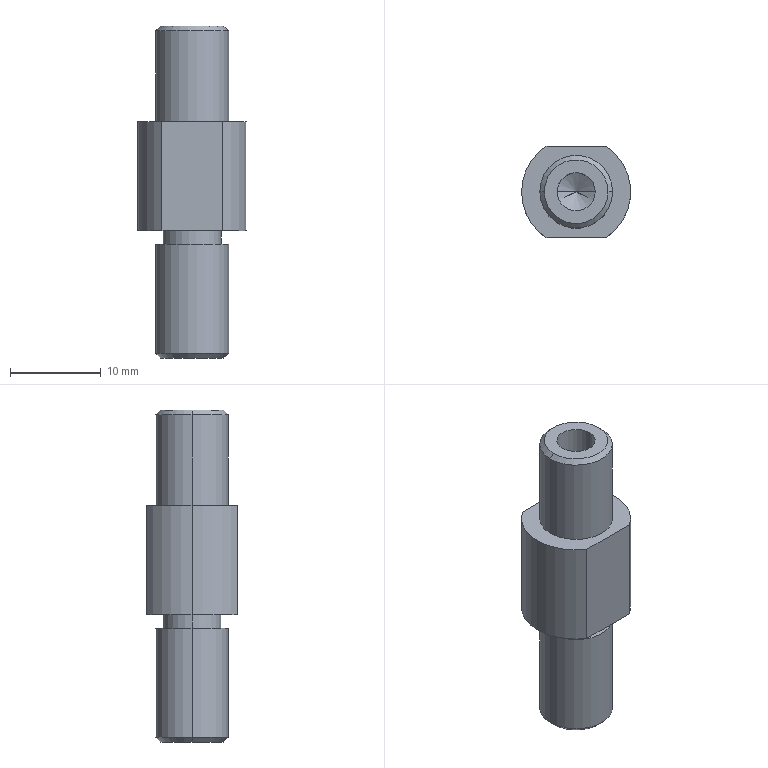Part | STEP file | 2014 Bag feed hold-down pivot shaft | 1 solid | 24 faces | box 12 x 10 x 36.5 mm | volume 2248 mm3 | cylinder 11 | plane 7 | cone 6 | commonest cylinder face diameters 8 x4 12 x3 4.2 x2 6.4 x2
STEP:
#1=CARTESIAN_POINT('',(0.,0.,0.));
#2=DIRECTION('',(0.,0.,1.));
#3=DIRECTION('',(1.,0.,0.));
#4=AXIS2_PLACEMENT_3D('',#1,#2,#3);
#5=CARTESIAN_POINT('',(4.,0.,-13.5));
#6=VERTEX_POINT('',#5);
#7=CARTESIAN_POINT('',(-4.,0.,-13.5));
#8=VERTEX_POINT('',#7);
#9=CARTESIAN_POINT('',(0.,0.,-13.5));
#10=DIRECTION('',(0.,0.,1.));
#11=DIRECTION('',(-1.,0.,0.));
#12=AXIS2_PLACEMENT_3D('',#9,#10,#11);
#13=CIRCLE('',#12,4.);
#14=CARTESIAN_POINT('',(0.,0.,-14.));
#15=DIRECTION('',(0.,0.,1.));
#16=DIRECTION('',(1.,0.,0.));
#17=AXIS2_PLACEMENT_3D('',#14,#15,#16);
#18=CYLINDRICAL_SURFACE('',#17,4.);
#19=CARTESIAN_POINT('',(-3.142,0.5));
#20=DIRECTION('',(1.,0.));
#21=VECTOR('',#20,1.);
#22=LINE('',#19,#21);
#23=(GEOMETRIC_REPRESENTATION_CONTEXT(2)PARAMETRIC_REPRESENTATION_CONTEXT()REPRESENTATION_CONTEXT('',''));
#24=DEFINITIONAL_REPRESENTATION('',(#22),#23);
#25=PCURVE('',#18,#24);
#26=CARTESIAN_POINT('',(0.,0.,-14.));
#27=DIRECTION('',(0.,0.,1.));
#28=DIRECTION('',(1.,0.,0.));
#29=AXIS2_PLACEMENT_3D('',#26,#27,#28);
#30=CONICAL_SURFACE('',#29,3.5,0.7854);
#31=CARTESIAN_POINT('',(-3.142,0.5));
#32=DIRECTION('',(1.,0.));
#33=VECTOR('',#32,1.);
#34=LINE('',#31,#33);
#35=(GEOMETRIC_REPRESENTATION_CONTEXT(2)PARAMETRIC_REPRESENTATION_CONTEXT()REPRESENTATION_CONTEXT('',''));
#36=DEFINITIONAL_REPRESENTATION('',(#34),#35);
#37=PCURVE('',#30,#36);
#38=SURFACE_CURVE('',#13,(#25,#37),.PCURVE_S1.);
#39=EDGE_CURVE('',#6,#8,#38,.T.);
#40=ORIENTED_EDGE('',*,*,#39,.T.);
#41=CARTESIAN_POINT('',(-4.,0.,-1.5));
#42=VERTEX_POINT('',#41);
#43=CARTESIAN_POINT('',(-4.,0.,-14.));
#44=DIRECTION('',(0.,0.,1.));
#45=VECTOR('',#44,1.);
#46=LINE('',#43,#45);
#47=CARTESIAN_POINT('',(3.142,0.));
#48=DIRECTION('',(0.,1.));
#49=VECTOR('',#48,1.);
#50=LINE('',#47,#49);
#51=(GEOMETRIC_REPRESENTATION_CONTEXT(2)PARAMETRIC_REPRESENTATION_CONTEXT()REPRESENTATION_CONTEXT('',''));
#52=DEFINITIONAL_REPRESENTATION('',(#50),#51);
#53=PCURVE('',#18,#52);
#54=CARTESIAN_POINT('',(0.,0.,-14.));
#55=DIRECTION('',(0.,0.,1.));
#56=DIRECTION('',(1.,0.,0.));
#57=AXIS2_PLACEMENT_3D('',#54,#55,#56);
#58=CYLINDRICAL_SURFACE('',#57,4.);
#59=CARTESIAN_POINT('',(3.142,0.));
#60=DIRECTION('',(0.,1.));
#61=VECTOR('',#60,1.);
#62=LINE('',#59,#61);
#63=(GEOMETRIC_REPRESENTATION_CONTEXT(2)PARAMETRIC_REPRESENTATION_CONTEXT()REPRESENTATION_CONTEXT('',''));
#64=DEFINITIONAL_REPRESENTATION('',(#62),#63);
#65=PCURVE('',#58,#64);
#66=SURFACE_CURVE('',#46,(#53,#65),.PCURVE_S1.);
#67=EDGE_CURVE('',#8,#42,#66,.T.);
#68=ORIENTED_EDGE('',*,*,#67,.T.);
#69=CARTESIAN_POINT('',(4.,0.,-1.5));
#70=VERTEX_POINT('',#69);
#71=CARTESIAN_POINT('',(0.,0.,-1.5));
#72=DIRECTION('',(0.,0.,-1.));
#73=DIRECTION('',(-1.,0.,0.));
#74=AXIS2_PLACEMENT_3D('',#71,#72,#73);
#75=CIRCLE('',#74,4.);
#76=CARTESIAN_POINT('',(3.142,12.5));
#77=DIRECTION('',(-1.,0.));
#78=VECTOR('',#77,1.);
#79=LINE('',#76,#78);
#80=(GEOMETRIC_REPRESENTATION_CONTEXT(2)PARAMETRIC_REPRESENTATION_CONTEXT()REPRESENTATION_CONTEXT('',''));
#81=DEFINITIONAL_REPRESENTATION('',(#79),#80);
#82=PCURVE('',#18,#81);
#83=CARTESIAN_POINT('',(-4.,0.,-1.5));
#84=DIRECTION('',(0.,0.,-1.));
#85=DIRECTION('',(-1.,0.,0.));
#86=AXIS2_PLACEMENT_3D('',#83,#84,#85);
#87=PLANE('',#86);
#88=CARTESIAN_POINT('',(-4.,0.));
#89=DIRECTION('',(1.,0.));
#90=AXIS2_PLACEMENT_2D('',#88,#89);
#91=CIRCLE('',#90,4.);
#92=(GEOMETRIC_REPRESENTATION_CONTEXT(2)PARAMETRIC_REPRESENTATION_CONTEXT()REPRESENTATION_CONTEXT('',''));
#93=DEFINITIONAL_REPRESENTATION('',(#91),#92);
#94=PCURVE('',#87,#93);
#95=SURFACE_CURVE('',#75,(#82,#94),.PCURVE_S1.);
#96=EDGE_CURVE('',#42,#70,#95,.T.);
#97=ORIENTED_EDGE('',*,*,#96,.T.);
#98=CARTESIAN_POINT('',(4.,0.,-14.));
#99=DIRECTION('',(0.,0.,1.));
#100=VECTOR('',#99,1.);
#101=LINE('',#98,#100);
#102=CARTESIAN_POINT('',(0.,0.));
#103=DIRECTION('',(0.,1.));
#104=VECTOR('',#103,1.);
#105=LINE('',#102,#104);
#106=(GEOMETRIC_REPRESENTATION_CONTEXT(2)PARAMETRIC_REPRESENTATION_CONTEXT()REPRESENTATION_CONTEXT('',''));
#107=DEFINITIONAL_REPRESENTATION('',(#105),#106);
#108=PCURVE('',#18,#107);
#109=CARTESIAN_POINT('',(6.283,0.));
#110=DIRECTION('',(0.,1.));
#111=VECTOR('',#110,1.);
#112=LINE('',#109,#111);
#113=(GEOMETRIC_REPRESENTATION_CONTEXT(2)PARAMETRIC_REPRESENTATION_CONTEXT()REPRESENTATION_CONTEXT('',''));
#114=DEFINITIONAL_REPRESENTATION('',(#112),#113);
#115=PCURVE('',#58,#114);
#116=SURFACE_CURVE('',#101,(#108,#115),.PCURVE_S1.);
#117=EDGE_CURVE('',#6,#70,#116,.T.);
#118=ORIENTED_EDGE('',*,*,#117,.F.);
#119=EDGE_LOOP('',(#40,#68,#97,#118));
#120=FACE_BOUND('',#119,.T.);
#121=ADVANCED_FACE('',(#120),#18,.T.);
#122=CARTESIAN_POINT('',(-3.5,0.,-14.));
#123=VERTEX_POINT('',#122);
#124=CARTESIAN_POINT('',(3.5,0.,-14.));
#125=VERTEX_POINT('',#124);
#126=CARTESIAN_POINT('',(0.,0.,-14.));
#127=DIRECTION('',(0.,0.,-1.));
#128=DIRECTION('',(-1.,0.,0.));
#129=AXIS2_PLACEMENT_3D('',#126,#127,#128);
#130=CIRCLE('',#129,3.5);
#131=CARTESIAN_POINT('',(3.142,0.));
#132=DIRECTION('',(-1.,0.));
#133=VECTOR('',#132,1.);
#134=LINE('',#131,#133);
#135=(GEOMETRIC_REPRESENTATION_CONTEXT(2)PARAMETRIC_REPRESENTATION_CONTEXT()REPRESENTATION_CONTEXT('',''));
#136=DEFINITIONAL_REPRESENTATION('',(#134),#135);
#137=PCURVE('',#30,#136);
#138=CARTESIAN_POINT('',(0.,0.,-14.));
#139=DIRECTION('',(0.,0.,-1.));
#140=DIRECTION('',(-1.,0.,0.));
#141=AXIS2_PLACEMENT_3D('',#138,#139,#140);
#142=PLANE('',#141);
#143=CARTESIAN_POINT('',(0.,0.));
#144=DIRECTION('',(1.,0.));
#145=AXIS2_PLACEMENT_2D('',#143,#144);
#146=CIRCLE('',#145,3.5);
#147=(GEOMETRIC_REPRESENTATION_CONTEXT(2)PARAMETRIC_REPRESENTATION_CONTEXT()REPRESENTATION_CONTEXT('',''));
#148=DEFINITIONAL_REPRESENTATION('',(#146),#147);
#149=PCURVE('',#142,#148);
#150=SURFACE_CURVE('',#130,(#137,#149),.PCURVE_S1.);
#151=EDGE_CURVE('',#123,#125,#150,.T.);
#152=ORIENTED_EDGE('',*,*,#151,.F.);
#153=CARTESIAN_POINT('',(-3.5,0.,-14.));
#154=DIRECTION('',(-0.7071,0.,0.7071));
#155=VECTOR('',#154,1.);
#156=LINE('',#153,#155);
#157=CARTESIAN_POINT('',(3.142,0.));
#158=DIRECTION('',(0.,1.));
#159=VECTOR('',#158,1.);
#160=LINE('',#157,#159);
#161=(GEOMETRIC_REPRESENTATION_CONTEXT(2)PARAMETRIC_REPRESENTATION_CONTEXT()REPRESENTATION_CONTEXT('',''));
#162=DEFINITIONAL_REPRESENTATION('',(#160),#161);
#163=PCURVE('',#30,#162);
#164=CARTESIAN_POINT('',(0.,0.,-14.));
#165=DIRECTION('',(0.,0.,1.));
#166=DIRECTION('',(1.,0.,0.));
#167=AXIS2_PLACEMENT_3D('',#164,#165,#166);
#168=CONICAL_SURFACE('',#167,3.5,0.7854);
#169=CARTESIAN_POINT('',(3.142,0.));
#170=DIRECTION('',(0.,1.));
#171=VECTOR('',#170,1.);
#172=LINE('',#169,#171);
#173=(GEOMETRIC_REPRESENTATION_CONTEXT(2)PARAMETRIC_REPRESENTATION_CONTEXT()REPRESENTATION_CONTEXT('',''));
#174=DEFINITIONAL_REPRESENTATION('',(#172),#173);
#175=PCURVE('',#168,#174);
#176=SURFACE_CURVE('',#156,(#163,#175),.PCURVE_S1.);
#177=EDGE_CURVE('',#123,#8,#176,.T.);
#178=ORIENTED_EDGE('',*,*,#177,.T.);
#179=ORIENTED_EDGE('',*,*,#39,.F.);
#180=CARTESIAN_POINT('',(3.5,0.,-14.));
#181=DIRECTION('',(0.7071,0.,0.7071));
#182=VECTOR('',#181,1.);
#183=LINE('',#180,#182);
#184=CARTESIAN_POINT('',(0.,0.));
#185=DIRECTION('',(0.,1.));
#186=VECTOR('',#185,1.);
#187=LINE('',#184,#186);
#188=(GEOMETRIC_REPRESENTATION_CONTEXT(2)PARAMETRIC_REPRESENTATION_CONTEXT()REPRESENTATION_CONTEXT('',''));
#189=DEFINITIONAL_REPRESENTATION('',(#187),#188);
#190=PCURVE('',#30,#189);
#191=CARTESIAN_POINT('',(6.283,0.));
#192=DIRECTION('',(0.,1.));
#193=VECTOR('',#192,1.);
#194=LINE('',#191,#193);
#195=(GEOMETRIC_REPRESENTATION_CONTEXT(2)PARAMETRIC_REPRESENTATION_CONTEXT()REPRESENTATION_CONTEXT('',''));
#196=DEFINITIONAL_REPRESENTATION('',(#194),#195);
#197=PCURVE('',#168,#196);
#198=SURFACE_CURVE('',#183,(#190,#197),.PCURVE_S1.);
#199=EDGE_CURVE('',#125,#6,#198,.T.);
#200=ORIENTED_EDGE('',*,*,#199,.F.);
#201=EDGE_LOOP('',(#152,#178,#179,#200));
#202=FACE_BOUND('',#201,.T.);
#203=ADVANCED_FACE('',(#202),#30,.T.);
#204=CARTESIAN_POINT('',(-3.2,0.,0.));
#205=VERTEX_POINT('',#204);
#206=CARTESIAN_POINT('',(3.2,0.,0.));
#207=VERTEX_POINT('',#206);
#208=CARTESIAN_POINT('',(0.,0.,0.));
#209=DIRECTION('',(0.,0.,-1.));
#210=DIRECTION('',(-1.,0.,0.));
#211=AXIS2_PLACEMENT_3D('',#208,#209,#210);
#212=CIRCLE('',#211,3.2);
#213=CARTESIAN_POINT('',(0.,0.,-13.5));
#214=DIRECTION('',(0.,0.,-1.));
#215=DIRECTION('',(-1.,0.,0.));
#216=AXIS2_PLACEMENT_3D('',#213,#214,#215);
#217=CYLINDRICAL_SURFACE('',#216,3.2);
#218=CARTESIAN_POINT('',(0.,-13.5));
#219=DIRECTION('',(1.,0.));
#220=VECTOR('',#219,1.);
#221=LINE('',#218,#220);
#222=(GEOMETRIC_REPRESENTATION_CONTEXT(2)PARAMETRIC_REPRESENTATION_CONTEXT()REPRESENTATION_CONTEXT('',''));
#223=DEFINITIONAL_REPRESENTATION('',(#221),#222);
#224=PCURVE('',#217,#223);
#225=CARTESIAN_POINT('',(0.,0.,0.));
#226=DIRECTION('',(0.,0.,1.));
#227=DIRECTION('',(1.,0.,0.));
#228=AXIS2_PLACEMENT_3D('',#225,#226,#227);
#229=PLANE('',#228);
#230=CARTESIAN_POINT('',(-3.2,0.));
#231=CARTESIAN_POINT('',(-3.2,5.543));
#232=CARTESIAN_POINT('',(1.6,2.771));
#233=CARTESIAN_POINT('',(6.4,0.));
#234=CARTESIAN_POINT('',(1.6,-2.771));
#235=CARTESIAN_POINT('',(-3.2,-5.543));
#236=CARTESIAN_POINT('',(-3.2,0.));
#237=(BOUNDED_CURVE()B_SPLINE_CURVE(2,(#230,#231,#232,#233,#234,#235,#236),.UNSPECIFIED.,.T.,.F.)B_SPLINE_CURVE_WITH_KNOTS((1,2,2,2,2,1),(-2.094,0.,2.094,4.189,6.283,8.378),.UNSPECIFIED.)CURVE()GEOMETRIC_REPRESENTATION_ITEM()RATIONAL_B_SPLINE_CURVE((1.,0.5,1.,0.5,1.,0.5,1.))REPRESENTATION_ITEM(''));
#238=(GEOMETRIC_REPRESENTATION_CONTEXT(2)PARAMETRIC_REPRESENTATION_CONTEXT()REPRESENTATION_CONTEXT('',''));
#239=DEFINITIONAL_REPRESENTATION('',(#237),#238);
#240=PCURVE('',#229,#239);
#241=SURFACE_CURVE('',#212,(#224,#240),.PCURVE_S1.);
#242=EDGE_CURVE('',#205,#207,#241,.T.);
#243=ORIENTED_EDGE('',*,*,#242,.T.);
#244=CARTESIAN_POINT('',(3.2,0.,-1.5));
#245=VERTEX_POINT('',#244);
#246=CARTESIAN_POINT('',(3.2,0.,-13.5));
#247=DIRECTION('',(0.,0.,-1.));
#248=VECTOR('',#247,1.);
#249=LINE('',#246,#248);
#250=CARTESIAN_POINT('',(3.142,0.));
#251=DIRECTION('',(0.,1.));
#252=VECTOR('',#251,1.);
#253=LINE('',#250,#252);
#254=(GEOMETRIC_REPRESENTATION_CONTEXT(2)PARAMETRIC_REPRESENTATION_CONTEXT()REPRESENTATION_CONTEXT('',''));
#255=DEFINITIONAL_REPRESENTATION('',(#253),#254);
#256=PCURVE('',#217,#255);
#257=CARTESIAN_POINT('',(0.,0.,-13.5));
#258=DIRECTION('',(0.,0.,-1.));
#259=DIRECTION('',(-1.,0.,0.));
#260=AXIS2_PLACEMENT_3D('',#257,#258,#259);
#261=CYLINDRICAL_SURFACE('',#260,3.2);
#262=CARTESIAN_POINT('',(3.142,0.));
#263=DIRECTION('',(0.,1.));
#264=VECTOR('',#263,1.);
#265=LINE('',#262,#264);
#266=(GEOMETRIC_REPRESENTATION_CONTEXT(2)PARAMETRIC_REPRESENTATION_CONTEXT()REPRESENTATION_CONTEXT('',''));
#267=DEFINITIONAL_REPRESENTATION('',(#265),#266);
#268=PCURVE('',#261,#267);
#269=SURFACE_CURVE('',#249,(#256,#268),.PCURVE_S1.);
#270=EDGE_CURVE('',#207,#245,#269,.T.);
#271=ORIENTED_EDGE('',*,*,#270,.T.);
#272=CARTESIAN_POINT('',(-3.2,0.,-1.5));
#273=VERTEX_POINT('',#272);
#274=CARTESIAN_POINT('',(0.,0.,-1.5));
#275=DIRECTION('',(0.,0.,-1.));
#276=DIRECTION('',(-1.,0.,0.));
#277=AXIS2_PLACEMENT_3D('',#274,#275,#276);
#278=CIRCLE('',#277,3.2);
#279=CARTESIAN_POINT('',(0.,-12.));
#280=DIRECTION('',(1.,0.));
#281=VECTOR('',#280,1.);
#282=LINE('',#279,#281);
#283=(GEOMETRIC_REPRESENTATION_CONTEXT(2)PARAMETRIC_REPRESENTATION_CONTEXT()REPRESENTATION_CONTEXT('',''));
#284=DEFINITIONAL_REPRESENTATION('',(#282),#283);
#285=PCURVE('',#217,#284);
#286=CARTESIAN_POINT('',(-4.,0.));
#287=DIRECTION('',(1.,0.));
#288=AXIS2_PLACEMENT_2D('',#286,#287);
#289=CIRCLE('',#288,3.2);
#290=(GEOMETRIC_REPRESENTATION_CONTEXT(2)PARAMETRIC_REPRESENTATION_CONTEXT()REPRESENTATION_CONTEXT('',''));
#291=DEFINITIONAL_REPRESENTATION('',(#289),#290);
#292=PCURVE('',#87,#291);
#293=SURFACE_CURVE('',#278,(#285,#292),.PCURVE_S1.);
#294=EDGE_CURVE('',#273,#245,#293,.T.);
#295=ORIENTED_EDGE('',*,*,#294,.F.);
#296=CARTESIAN_POINT('',(-3.2,0.,-13.5));
#297=DIRECTION('',(0.,0.,-1.));
#298=VECTOR('',#297,1.);
#299=LINE('',#296,#298);
#300=CARTESIAN_POINT('',(0.,0.));
#301=DIRECTION('',(0.,1.));
#302=VECTOR('',#301,1.);
#303=LINE('',#300,#302);
#304=(GEOMETRIC_REPRESENTATION_CONTEXT(2)PARAMETRIC_REPRESENTATION_CONTEXT()REPRESENTATION_CONTEXT('',''));
#305=DEFINITIONAL_REPRESENTATION('',(#303),#304);
#306=PCURVE('',#217,#305);
#307=CARTESIAN_POINT('',(6.283,0.));
#308=DIRECTION('',(0.,1.));
#309=VECTOR('',#308,1.);
#310=LINE('',#307,#309);
#311=(GEOMETRIC_REPRESENTATION_CONTEXT(2)PARAMETRIC_REPRESENTATION_CONTEXT()REPRESENTATION_CONTEXT('',''));
#312=DEFINITIONAL_REPRESENTATION('',(#310),#311);
#313=PCURVE('',#261,#312);
#314=SURFACE_CURVE('',#299,(#306,#313),.PCURVE_S1.);
#315=EDGE_CURVE('',#205,#273,#314,.T.);
#316=ORIENTED_EDGE('',*,*,#315,.F.);
#317=EDGE_LOOP('',(#243,#271,#295,#316));
#318=FACE_BOUND('',#317,.T.);
#319=ADVANCED_FACE('',(#318),#217,.T.);
#320=CARTESIAN_POINT('',(3.5,0.,22.5));
#321=VERTEX_POINT('',#320);
#322=CARTESIAN_POINT('',(-3.5,0.,22.5));
#323=VERTEX_POINT('',#322);
#324=CARTESIAN_POINT('',(0.,0.,22.5));
#325=DIRECTION('',(0.,0.,1.));
#326=DIRECTION('',(1.,0.,0.));
#327=AXIS2_PLACEMENT_3D('',#324,#325,#326);
#328=CIRCLE('',#327,3.5);
#329=CARTESIAN_POINT('',(0.,0.,22.5));
#330=DIRECTION('',(0.,0.,-1.));
#331=DIRECTION('',(-1.,0.,0.));
#332=AXIS2_PLACEMENT_3D('',#329,#330,#331);
#333=CONICAL_SURFACE('',#332,3.5,0.7854);
#334=CARTESIAN_POINT('',(3.142,0.));
#335=DIRECTION('',(-1.,0.));
#336=VECTOR('',#335,1.);
#337=LINE('',#334,#336);
#338=(GEOMETRIC_REPRESENTATION_CONTEXT(2)PARAMETRIC_REPRESENTATION_CONTEXT()REPRESENTATION_CONTEXT('',''));
#339=DEFINITIONAL_REPRESENTATION('',(#337),#338);
#340=PCURVE('',#333,#339);
#341=CARTESIAN_POINT('',(0.,0.,22.5));
#342=DIRECTION('',(0.,0.,1.));
#343=DIRECTION('',(1.,0.,0.));
#344=AXIS2_PLACEMENT_3D('',#341,#342,#343);
#345=PLANE('',#344);
#346=CARTESIAN_POINT('',(0.,0.));
#347=DIRECTION('',(1.,0.));
#348=AXIS2_PLACEMENT_2D('',#346,#347);
#349=CIRCLE('',#348,3.5);
#350=(GEOMETRIC_REPRESENTATION_CONTEXT(2)PARAMETRIC_REPRESENTATION_CONTEXT()REPRESENTATION_CONTEXT('',''));
#351=DEFINITIONAL_REPRESENTATION('',(#349),#350);
#352=PCURVE('',#345,#351);
#353=SURFACE_CURVE('',#328,(#340,#352),.PCURVE_S1.);
#354=EDGE_CURVE('',#321,#323,#353,.T.);
#355=ORIENTED_EDGE('',*,*,#354,.F.);
#356=CARTESIAN_POINT('',(4.,0.,22.));
#357=VERTEX_POINT('',#356);
#358=CARTESIAN_POINT('',(3.5,0.,22.5));
#359=DIRECTION('',(0.7071,0.,-0.7071));
#360=VECTOR('',#359,1.);
#361=LINE('',#358,#360);
#362=CARTESIAN_POINT('',(3.142,0.));
#363=DIRECTION('',(0.,1.));
#364=VECTOR('',#363,1.);
#365=LINE('',#362,#364);
#366=(GEOMETRIC_REPRESENTATION_CONTEXT(2)PARAMETRIC_REPRESENTATION_CONTEXT()REPRESENTATION_CONTEXT('',''));
#367=DEFINITIONAL_REPRESENTATION('',(#365),#366);
#368=PCURVE('',#333,#367);
#369=CARTESIAN_POINT('',(0.,0.,22.5));
#370=DIRECTION('',(0.,0.,-1.));
#371=DIRECTION('',(-1.,0.,0.));
#372=AXIS2_PLACEMENT_3D('',#369,#370,#371);
#373=CONICAL_SURFACE('',#372,3.5,0.7854);
#374=CARTESIAN_POINT('',(3.142,0.));
#375=DIRECTION('',(0.,1.));
#376=VECTOR('',#375,1.);
#377=LINE('',#374,#376);
#378=(GEOMETRIC_REPRESENTATION_CONTEXT(2)PARAMETRIC_REPRESENTATION_CONTEXT()REPRESENTATION_CONTEXT('',''));
#379=DEFINITIONAL_REPRESENTATION('',(#377),#378);
#380=PCURVE('',#373,#379);
#381=SURFACE_CURVE('',#361,(#368,#380),.PCURVE_S1.);
#382=EDGE_CURVE('',#321,#357,#381,.T.);
#383=ORIENTED_EDGE('',*,*,#382,.T.);
#384=CARTESIAN_POINT('',(-4.,0.,22.));
#385=VERTEX_POINT('',#384);
#386=CARTESIAN_POINT('',(0.,0.,22.));
#387=DIRECTION('',(0.,0.,-1.));
#388=DIRECTION('',(1.,0.,0.));
#389=AXIS2_PLACEMENT_3D('',#386,#387,#388);
#390=CIRCLE('',#389,4.);
#391=CARTESIAN_POINT('',(-3.142,0.5));
#392=DIRECTION('',(1.,0.));
#393=VECTOR('',#392,1.);
#394=LINE('',#391,#393);
#395=(GEOMETRIC_REPRESENTATION_CONTEXT(2)PARAMETRIC_REPRESENTATION_CONTEXT()REPRESENTATION_CONTEXT('',''));
#396=DEFINITIONAL_REPRESENTATION('',(#394),#395);
#397=PCURVE('',#333,#396);
#398=CARTESIAN_POINT('',(0.,0.,22.5));
#399=DIRECTION('',(0.,0.,-1.));
#400=DIRECTION('',(-1.,0.,0.));
#401=AXIS2_PLACEMENT_3D('',#398,#399,#400);
#402=CYLINDRICAL_SURFACE('',#401,4.);
#403=CARTESIAN_POINT('',(-3.142,0.5));
#404=DIRECTION('',(1.,0.));
#405=VECTOR('',#404,1.);
#406=LINE('',#403,#405);
#407=(GEOMETRIC_REPRESENTATION_CONTEXT(2)PARAMETRIC_REPRESENTATION_CONTEXT()REPRESENTATION_CONTEXT('',''));
#408=DEFINITIONAL_REPRESENTATION('',(#406),#407);
#409=PCURVE('',#402,#408);
#410=SURFACE_CURVE('',#390,(#397,#409),.PCURVE_S1.);
#411=EDGE_CURVE('',#385,#357,#410,.T.);
#412=ORIENTED_EDGE('',*,*,#411,.F.);
#413=CARTESIAN_POINT('',(-3.5,0.,22.5));
#414=DIRECTION('',(-0.7071,0.,-0.7071));
#415=VECTOR('',#414,1.);
#416=LINE('',#413,#415);
#417=CARTESIAN_POINT('',(0.,0.));
#418=DIRECTION('',(0.,1.));
#419=VECTOR('',#418,1.);
#420=LINE('',#417,#419);
#421=(GEOMETRIC_REPRESENTATION_CONTEXT(2)PARAMETRIC_REPRESENTATION_CONTEXT()REPRESENTATION_CONTEXT('',''));
#422=DEFINITIONAL_REPRESENTATION('',(#420),#421);
#423=PCURVE('',#333,#422);
#424=CARTESIAN_POINT('',(6.283,0.));
#425=DIRECTION('',(0.,1.));
#426=VECTOR('',#425,1.);
#427=LINE('',#424,#426);
#428=(GEOMETRIC_REPRESENTATION_CONTEXT(2)PARAMETRIC_REPRESENTATION_CONTEXT()REPRESENTATION_CONTEXT('',''));
#429=DEFINITIONAL_REPRESENTATION('',(#427),#428);
#430=PCURVE('',#373,#429);
#431=SURFACE_CURVE('',#416,(#423,#430),.PCURVE_S1.);
#432=EDGE_CURVE('',#323,#385,#431,.T.);
#433=ORIENTED_EDGE('',*,*,#432,.F.);
#434=EDGE_LOOP('',(#355,#383,#412,#433));
#435=FACE_BOUND('',#434,.T.);
#436=ADVANCED_FACE('',(#435),#333,.T.);
#437=CARTESIAN_POINT('',(2.1,0.,8.5));
#438=VERTEX_POINT('',#437);
#439=CARTESIAN_POINT('',(2.1,0.,22.5));
#440=VERTEX_POINT('',#439);
#441=CARTESIAN_POINT('',(2.1,0.,22.5));
#442=DIRECTION('',(0.,0.,1.));
#443=VECTOR('',#442,1.);
#444=LINE('',#441,#443);
#445=CARTESIAN_POINT('',(0.,0.,22.5));
#446=DIRECTION('',(0.,0.,1.));
#447=DIRECTION('',(1.,0.,0.));
#448=AXIS2_PLACEMENT_3D('',#445,#446,#447);
#449=CYLINDRICAL_SURFACE('',#448,2.1);
#450=CARTESIAN_POINT('',(6.283,0.));
#451=DIRECTION('',(0.,1.));
#452=VECTOR('',#451,1.);
#453=LINE('',#450,#452);
#454=(GEOMETRIC_REPRESENTATION_CONTEXT(2)PARAMETRIC_REPRESENTATION_CONTEXT()REPRESENTATION_CONTEXT('',''));
#455=DEFINITIONAL_REPRESENTATION('',(#453),#454);
#456=PCURVE('',#449,#455);
#457=CARTESIAN_POINT('',(0.,0.,22.5));
#458=DIRECTION('',(0.,0.,1.));
#459=DIRECTION('',(1.,0.,0.));
#460=AXIS2_PLACEMENT_3D('',#457,#458,#459);
#461=CYLINDRICAL_SURFACE('',#460,2.1);
#462=CARTESIAN_POINT('',(0.,0.));
#463=DIRECTION('',(0.,1.));
#464=VECTOR('',#463,1.);
#465=LINE('',#462,#464);
#466=(GEOMETRIC_REPRESENTATION_CONTEXT(2)PARAMETRIC_REPRESENTATION_CONTEXT()REPRESENTATION_CONTEXT('',''));
#467=DEFINITIONAL_REPRESENTATION('',(#465),#466);
#468=PCURVE('',#461,#467);
#469=SURFACE_CURVE('',#444,(#456,#468),.PCURVE_S1.);
#470=EDGE_CURVE('',#438,#440,#469,.T.);
#471=ORIENTED_EDGE('',*,*,#470,.T.);
#472=CARTESIAN_POINT('',(-2.1,0.,22.5));
#473=VERTEX_POINT('',#472);
#474=CARTESIAN_POINT('',(0.,0.,22.5));
#475=DIRECTION('',(0.,0.,1.));
#476=DIRECTION('',(1.,0.,0.));
#477=AXIS2_PLACEMENT_3D('',#474,#475,#476);
#478=CIRCLE('',#477,2.1);
#479=CARTESIAN_POINT('',(0.,0.));
#480=DIRECTION('',(1.,0.));
#481=VECTOR('',#480,1.);
#482=LINE('',#479,#481);
#483=(GEOMETRIC_REPRESENTATION_CONTEXT(2)PARAMETRIC_REPRESENTATION_CONTEXT()REPRESENTATION_CONTEXT('',''));
#484=DEFINITIONAL_REPRESENTATION('',(#482),#483);
#485=PCURVE('',#449,#484);
#486=CARTESIAN_POINT('',(0.,0.));
#487=DIRECTION('',(1.,0.));
#488=AXIS2_PLACEMENT_2D('',#486,#487);
#489=CIRCLE('',#488,2.1);
#490=(GEOMETRIC_REPRESENTATION_CONTEXT(2)PARAMETRIC_REPRESENTATION_CONTEXT()REPRESENTATION_CONTEXT('',''));
#491=DEFINITIONAL_REPRESENTATION('',(#489),#490);
#492=PCURVE('',#345,#491);
#493=SURFACE_CURVE('',#478,(#485,#492),.PCURVE_S1.);
#494=EDGE_CURVE('',#473,#440,#493,.T.);
#495=ORIENTED_EDGE('',*,*,#494,.F.);
#496=CARTESIAN_POINT('',(-2.1,0.,8.5));
#497=VERTEX_POINT('',#496);
#498=CARTESIAN_POINT('',(-2.1,0.,22.5));
#499=DIRECTION('',(0.,0.,1.));
#500=VECTOR('',#499,1.);
#501=LINE('',#498,#500);
#502=CARTESIAN_POINT('',(3.142,0.));
#503=DIRECTION('',(0.,1.));
#504=VECTOR('',#503,1.);
#505=LINE('',#502,#504);
#506=(GEOMETRIC_REPRESENTATION_CONTEXT(2)PARAMETRIC_REPRESENTATION_CONTEXT()REPRESENTATION_CONTEXT('',''));
#507=DEFINITIONAL_REPRESENTATION('',(#505),#506);
#508=PCURVE('',#449,#507);
#509=CARTESIAN_POINT('',(3.142,0.));
#510=DIRECTION('',(0.,1.));
#511=VECTOR('',#510,1.);
#512=LINE('',#509,#511);
#513=(GEOMETRIC_REPRESENTATION_CONTEXT(2)PARAMETRIC_REPRESENTATION_CONTEXT()REPRESENTATION_CONTEXT('',''));
#514=DEFINITIONAL_REPRESENTATION('',(#512),#513);
#515=PCURVE('',#461,#514);
#516=SURFACE_CURVE('',#501,(#508,#515),.PCURVE_S1.);
#517=EDGE_CURVE('',#497,#473,#516,.T.);
#518=ORIENTED_EDGE('',*,*,#517,.F.);
#519=CARTESIAN_POINT('',(0.,0.,8.5));
#520=DIRECTION('',(0.,0.,1.));
#521=DIRECTION('',(1.,0.,0.));
#522=AXIS2_PLACEMENT_3D('',#519,#520,#521);
#523=CIRCLE('',#522,2.1);
#524=CARTESIAN_POINT('',(0.,-14.));
#525=DIRECTION('',(1.,0.));
#526=VECTOR('',#525,1.);
#527=LINE('',#524,#526);
#528=(GEOMETRIC_REPRESENTATION_CONTEXT(2)PARAMETRIC_REPRESENTATION_CONTEXT()REPRESENTATION_CONTEXT('',''));
#529=DEFINITIONAL_REPRESENTATION('',(#527),#528);
#530=PCURVE('',#449,#529);
#531=CARTESIAN_POINT('',(0.,0.,8.5));
#532=DIRECTION('',(0.,0.,1.));
#533=DIRECTION('',(1.,0.,0.));
#534=AXIS2_PLACEMENT_3D('',#531,#532,#533);
#535=CONICAL_SURFACE('',#534,2.1,1.03);
#536=CARTESIAN_POINT('',(0.,0.));
#537=DIRECTION('',(1.,0.));
#538=VECTOR('',#537,1.);
#539=LINE('',#536,#538);
#540=(GEOMETRIC_REPRESENTATION_CONTEXT(2)PARAMETRIC_REPRESENTATION_CONTEXT()REPRESENTATION_CONTEXT('',''));
#541=DEFINITIONAL_REPRESENTATION('',(#539),#540);
#542=PCURVE('',#535,#541);
#543=SURFACE_CURVE('',#523,(#530,#542),.PCURVE_S1.);
#544=EDGE_CURVE('',#497,#438,#543,.T.);
#545=ORIENTED_EDGE('',*,*,#544,.T.);
#546=EDGE_LOOP('',(#471,#495,#518,#545));
#547=FACE_BOUND('',#546,.F.);
#548=ADVANCED_FACE('',(#547),#449,.F.);
#549=ORIENTED_EDGE('',*,*,#544,.F.);
#550=CARTESIAN_POINT('',(0.,0.,7.238));
#551=VERTEX_POINT('',#550);
#552=CARTESIAN_POINT('',(-2.1,0.,8.5));
#553=DIRECTION('',(-0.8572,0.,0.515));
#554=VECTOR('',#553,1.);
#555=LINE('',#552,#554);
#556=CARTESIAN_POINT('',(3.142,0.));
#557=DIRECTION('',(0.,1.));
#558=VECTOR('',#557,1.);
#559=LINE('',#556,#558);
#560=(GEOMETRIC_REPRESENTATION_CONTEXT(2)PARAMETRIC_REPRESENTATION_CONTEXT()REPRESENTATION_CONTEXT('',''));
#561=DEFINITIONAL_REPRESENTATION('',(#559),#560);
#562=PCURVE('',#535,#561);
#563=CARTESIAN_POINT('',(0.,0.,8.5));
#564=DIRECTION('',(0.,0.,1.));
#565=DIRECTION('',(1.,0.,0.));
#566=AXIS2_PLACEMENT_3D('',#563,#564,#565);
#567=CONICAL_SURFACE('',#566,2.1,1.03);
#568=CARTESIAN_POINT('',(3.142,0.));
#569=DIRECTION('',(0.,1.));
#570=VECTOR('',#569,1.);
#571=LINE('',#568,#570);
#572=(GEOMETRIC_REPRESENTATION_CONTEXT(2)PARAMETRIC_REPRESENTATION_CONTEXT()REPRESENTATION_CONTEXT('',''));
#573=DEFINITIONAL_REPRESENTATION('',(#571),#572);
#574=PCURVE('',#567,#573);
#575=SURFACE_CURVE('',#555,(#562,#574),.PCURVE_S1.);
#576=EDGE_CURVE('',#551,#497,#575,.T.);
#577=ORIENTED_EDGE('',*,*,#576,.F.);
#578=CARTESIAN_POINT('',(2.1,0.,8.5));
#579=DIRECTION('',(0.8572,0.,0.515));
#580=VECTOR('',#579,1.);
#581=LINE('',#578,#580);
#582=CARTESIAN_POINT('',(6.283,-1.262));
#583=CARTESIAN_POINT('',(6.283,-1.243));
#584=CARTESIAN_POINT('',(6.283,-1.204));
#585=CARTESIAN_POINT('',(6.283,-1.147));
#586=CARTESIAN_POINT('',(6.283,-1.09));
#587=CARTESIAN_POINT('',(6.283,-1.032));
#588=CARTESIAN_POINT('',(6.283,-0.975));
#589=CARTESIAN_POINT('',(6.283,-0.9177));
#590=CARTESIAN_POINT('',(6.283,-0.8603));
#591=CARTESIAN_POINT('',(6.283,-0.803));
#592=CARTESIAN_POINT('',(6.283,-0.7456));
#593=CARTESIAN_POINT('',(6.283,-0.6883));
#594=CARTESIAN_POINT('',(6.283,-0.6309));
#595=CARTESIAN_POINT('',(6.283,-0.5735));
#596=CARTESIAN_POINT('',(6.283,-0.5162));
#597=CARTESIAN_POINT('',(6.283,-0.4588));
#598=CARTESIAN_POINT('',(6.283,-0.4015));
#599=CARTESIAN_POINT('',(6.283,-0.3441));
#600=CARTESIAN_POINT('',(6.283,-0.2868));
#601=CARTESIAN_POINT('',(6.283,-0.2294));
#602=CARTESIAN_POINT('',(6.283,-0.1721));
#603=CARTESIAN_POINT('',(6.283,-0.1147));
#604=CARTESIAN_POINT('',(6.283,-0.05735));
#605=CARTESIAN_POINT('',(6.283,-0.01912));
#606=CARTESIAN_POINT('',(6.283,0.));
#607=B_SPLINE_CURVE_WITH_KNOTS('',3,(#582,#583,#584,#585,#586,#587,#588,#589,#590,#591,#592,#593,#594,#595,#596,#597,#598,#599,#600,#601,#602,#603,#604,#605,#606),.UNSPECIFIED.,.F.,.F.,(4,1,1,1,1,1,1,1,1,1,1,1,1,1,1,1,1,1,1,1,1,1,4),(-2.45,-2.339,-2.227,-2.116,-2.004,-1.893,-1.782,-1.67,-1.559,-1.448,-1.336,-1.225,-1.114,-1.002,-0.8909,-0.7795,-0.6682,-0.5568,-0.4454,-0.3341,-0.2227,-0.1114,0.),.QUASI_UNIFORM_KNOTS.);
#608=(GEOMETRIC_REPRESENTATION_CONTEXT(2)PARAMETRIC_REPRESENTATION_CONTEXT()REPRESENTATION_CONTEXT('',''));
#609=DEFINITIONAL_REPRESENTATION('',(#607),#608);
#610=PCURVE('',#535,#609);
#611=CARTESIAN_POINT('',(0.,-1.262));
#612=CARTESIAN_POINT('',(0.,-1.243));
#613=CARTESIAN_POINT('',(0.,-1.204));
#614=CARTESIAN_POINT('',(0.,-1.147));
#615=CARTESIAN_POINT('',(0.,-1.09));
#616=CARTESIAN_POINT('',(0.,-1.032));
#617=CARTESIAN_POINT('',(0.,-0.975));
#618=CARTESIAN_POINT('',(0.,-0.9177));
#619=CARTESIAN_POINT('',(0.,-0.8603));
#620=CARTESIAN_POINT('',(0.,-0.803));
#621=CARTESIAN_POINT('',(0.,-0.7456));
#622=CARTESIAN_POINT('',(0.,-0.6883));
#623=CARTESIAN_POINT('',(0.,-0.6309));
#624=CARTESIAN_POINT('',(0.,-0.5735));
#625=CARTESIAN_POINT('',(0.,-0.5162));
#626=CARTESIAN_POINT('',(0.,-0.4588));
#627=CARTESIAN_POINT('',(0.,-0.4015));
#628=CARTESIAN_POINT('',(0.,-0.3441));
#629=CARTESIAN_POINT('',(0.,-0.2868));
#630=CARTESIAN_POINT('',(0.,-0.2294));
#631=CARTESIAN_POINT('',(0.,-0.1721));
#632=CARTESIAN_POINT('',(0.,-0.1147));
#633=CARTESIAN_POINT('',(0.,-0.05735));
#634=CARTESIAN_POINT('',(0.,-0.01912));
#635=CARTESIAN_POINT('',(0.,0.));
#636=B_SPLINE_CURVE_WITH_KNOTS('',3,(#611,#612,#613,#614,#615,#616,#617,#618,#619,#620,#621,#622,#623,#624,#625,#626,#627,#628,#629,#630,#631,#632,#633,#634,#635),.UNSPECIFIED.,.F.,.F.,(4,1,1,1,1,1,1,1,1,1,1,1,1,1,1,1,1,1,1,1,1,1,4),(-2.45,-2.339,-2.227,-2.116,-2.004,-1.893,-1.782,-1.67,-1.559,-1.448,-1.336,-1.225,-1.114,-1.002,-0.8909,-0.7795,-0.6682,-0.5568,-0.4454,-0.3341,-0.2227,-0.1114,0.),.QUASI_UNIFORM_KNOTS.);
#637=(GEOMETRIC_REPRESENTATION_CONTEXT(2)PARAMETRIC_REPRESENTATION_CONTEXT()REPRESENTATION_CONTEXT('',''));
#638=DEFINITIONAL_REPRESENTATION('',(#636),#637);
#639=PCURVE('',#567,#638);
#640=SURFACE_CURVE('',#581,(#610,#639),.PCURVE_S1.);
#641=EDGE_CURVE('',#551,#438,#640,.T.);
#642=ORIENTED_EDGE('',*,*,#641,.T.);
#643=EDGE_LOOP('',(#549,#577,#642));
#644=FACE_BOUND('',#643,.F.);
#645=ADVANCED_FACE('',(#644),#535,.F.);
#646=ORIENTED_EDGE('',*,*,#411,.T.);
#647=CARTESIAN_POINT('',(4.,0.,12.));
#648=VERTEX_POINT('',#647);
#649=CARTESIAN_POINT('',(4.,0.,22.5));
#650=DIRECTION('',(0.,0.,-1.));
#651=VECTOR('',#650,1.);
#652=LINE('',#649,#651);
#653=CARTESIAN_POINT('',(3.142,0.));
#654=DIRECTION('',(0.,1.));
#655=VECTOR('',#654,1.);
#656=LINE('',#653,#655);
#657=(GEOMETRIC_REPRESENTATION_CONTEXT(2)PARAMETRIC_REPRESENTATION_CONTEXT()REPRESENTATION_CONTEXT('',''));
#658=DEFINITIONAL_REPRESENTATION('',(#656),#657);
#659=PCURVE('',#402,#658);
#660=CARTESIAN_POINT('',(0.,0.,22.5));
#661=DIRECTION('',(0.,0.,-1.));
#662=DIRECTION('',(-1.,0.,0.));
#663=AXIS2_PLACEMENT_3D('',#660,#661,#662);
#664=CYLINDRICAL_SURFACE('',#663,4.);
#665=CARTESIAN_POINT('',(3.142,0.));
#666=DIRECTION('',(0.,1.));
#667=VECTOR('',#666,1.);
#668=LINE('',#665,#667);
#669=(GEOMETRIC_REPRESENTATION_CONTEXT(2)PARAMETRIC_REPRESENTATION_CONTEXT()REPRESENTATION_CONTEXT('',''));
#670=DEFINITIONAL_REPRESENTATION('',(#668),#669);
#671=PCURVE('',#664,#670);
#672=SURFACE_CURVE('',#652,(#659,#671),.PCURVE_S1.);
#673=EDGE_CURVE('',#357,#648,#672,.T.);
#674=ORIENTED_EDGE('',*,*,#673,.T.);
#675=CARTESIAN_POINT('',(-4.,0.,12.));
#676=VERTEX_POINT('',#675);
#677=CARTESIAN_POINT('',(0.,0.,12.));
#678=DIRECTION('',(0.,0.,1.));
#679=DIRECTION('',(1.,0.,0.));
#680=AXIS2_PLACEMENT_3D('',#677,#678,#679);
#681=CIRCLE('',#680,4.);
#682=CARTESIAN_POINT('',(3.142,10.5));
#683=DIRECTION('',(-1.,0.));
#684=VECTOR('',#683,1.);
#685=LINE('',#682,#684);
#686=(GEOMETRIC_REPRESENTATION_CONTEXT(2)PARAMETRIC_REPRESENTATION_CONTEXT()REPRESENTATION_CONTEXT('',''));
#687=DEFINITIONAL_REPRESENTATION('',(#685),#686);
#688=PCURVE('',#402,#687);
#689=CARTESIAN_POINT('',(0.,0.,12.));
#690=DIRECTION('',(0.,0.,1.));
#691=DIRECTION('',(1.,0.,0.));
#692=AXIS2_PLACEMENT_3D('',#689,#690,#691);
#693=PLANE('',#692);
#694=CARTESIAN_POINT('',(0.,0.));
#695=DIRECTION('',(1.,0.));
#696=AXIS2_PLACEMENT_2D('',#694,#695);
#697=CIRCLE('',#696,4.);
#698=(GEOMETRIC_REPRESENTATION_CONTEXT(2)PARAMETRIC_REPRESENTATION_CONTEXT()REPRESENTATION_CONTEXT('',''));
#699=DEFINITIONAL_REPRESENTATION('',(#697),#698);
#700=PCURVE('',#693,#699);
#701=SURFACE_CURVE('',#681,(#688,#700),.PCURVE_S1.);
#702=EDGE_CURVE('',#648,#676,#701,.T.);
#703=ORIENTED_EDGE('',*,*,#702,.T.);
#704=CARTESIAN_POINT('',(-4.,0.,22.5));
#705=DIRECTION('',(0.,0.,-1.));
#706=VECTOR('',#705,1.);
#707=LINE('',#704,#706);
#708=CARTESIAN_POINT('',(0.,0.));
#709=DIRECTION('',(0.,1.));
#710=VECTOR('',#709,1.);
#711=LINE('',#708,#710);
#712=(GEOMETRIC_REPRESENTATION_CONTEXT(2)PARAMETRIC_REPRESENTATION_CONTEXT()REPRESENTATION_CONTEXT('',''));
#713=DEFINITIONAL_REPRESENTATION('',(#711),#712);
#714=PCURVE('',#402,#713);
#715=CARTESIAN_POINT('',(6.283,0.));
#716=DIRECTION('',(0.,1.));
#717=VECTOR('',#716,1.);
#718=LINE('',#715,#717);
#719=(GEOMETRIC_REPRESENTATION_CONTEXT(2)PARAMETRIC_REPRESENTATION_CONTEXT()REPRESENTATION_CONTEXT('',''));
#720=DEFINITIONAL_REPRESENTATION('',(#718),#719);
#721=PCURVE('',#664,#720);
#722=SURFACE_CURVE('',#707,(#714,#721),.PCURVE_S1.);
#723=EDGE_CURVE('',#385,#676,#722,.T.);
#724=ORIENTED_EDGE('',*,*,#723,.F.);
#725=EDGE_LOOP('',(#646,#674,#703,#724));
#726=FACE_BOUND('',#725,.T.);
#727=ADVANCED_FACE('',(#726),#402,.T.);
#728=CARTESIAN_POINT('',(-6.,0.,12.));
#729=VERTEX_POINT('',#728);
#730=CARTESIAN_POINT('',(-3.317,-5.,12.));
#731=VERTEX_POINT('',#730);
#732=CARTESIAN_POINT('',(0.,0.,12.));
#733=DIRECTION('',(0.,0.,1.));
#734=DIRECTION('',(1.,0.,0.));
#735=AXIS2_PLACEMENT_3D('',#732,#733,#734);
#736=CIRCLE('',#735,6.);
#737=CARTESIAN_POINT('',(0.,0.,12.));
#738=DIRECTION('',(0.,0.,-1.));
#739=DIRECTION('',(-1.,0.,0.));
#740=AXIS2_PLACEMENT_3D('',#737,#738,#739);
#741=CYLINDRICAL_SURFACE('',#740,6.);
#742=CARTESIAN_POINT('',(9.425,0.));
#743=DIRECTION('',(-1.,0.));
#744=VECTOR('',#743,1.);
#745=LINE('',#742,#744);
#746=(GEOMETRIC_REPRESENTATION_CONTEXT(2)PARAMETRIC_REPRESENTATION_CONTEXT()REPRESENTATION_CONTEXT('',''));
#747=DEFINITIONAL_REPRESENTATION('',(#745),#746);
#748=PCURVE('',#741,#747);
#749=CARTESIAN_POINT('',(0.,0.));
#750=DIRECTION('',(1.,0.));
#751=AXIS2_PLACEMENT_2D('',#749,#750);
#752=CIRCLE('',#751,6.);
#753=(GEOMETRIC_REPRESENTATION_CONTEXT(2)PARAMETRIC_REPRESENTATION_CONTEXT()REPRESENTATION_CONTEXT('',''));
#754=DEFINITIONAL_REPRESENTATION('',(#752),#753);
#755=PCURVE('',#693,#754);
#756=SURFACE_CURVE('',#736,(#748,#755),.PCURVE_S1.);
#757=EDGE_CURVE('',#729,#731,#756,.T.);
#758=ORIENTED_EDGE('',*,*,#757,.F.);
#759=CARTESIAN_POINT('',(-6.,0.,0.));
#760=VERTEX_POINT('',#759);
#761=CARTESIAN_POINT('',(-6.,0.,12.));
#762=DIRECTION('',(0.,0.,-1.));
#763=VECTOR('',#762,1.);
#764=LINE('',#761,#763);
#765=CARTESIAN_POINT('',(6.283,0.));
#766=DIRECTION('',(0.,1.));
#767=VECTOR('',#766,1.);
#768=LINE('',#765,#767);
#769=(GEOMETRIC_REPRESENTATION_CONTEXT(2)PARAMETRIC_REPRESENTATION_CONTEXT()REPRESENTATION_CONTEXT('',''));
#770=DEFINITIONAL_REPRESENTATION('',(#768),#769);
#771=PCURVE('',#741,#770);
#772=CARTESIAN_POINT('',(0.,0.,12.));
#773=DIRECTION('',(0.,0.,-1.));
#774=DIRECTION('',(-1.,0.,0.));
#775=AXIS2_PLACEMENT_3D('',#772,#773,#774);
#776=CYLINDRICAL_SURFACE('',#775,6.);
#777=CARTESIAN_POINT('',(0.,0.));
#778=DIRECTION('',(0.,1.));
#779=VECTOR('',#778,1.);
#780=LINE('',#777,#779);
#781=(GEOMETRIC_REPRESENTATION_CONTEXT(2)PARAMETRIC_REPRESENTATION_CONTEXT()REPRESENTATION_CONTEXT('',''));
#782=DEFINITIONAL_REPRESENTATION('',(#780),#781);
#783=PCURVE('',#776,#782);
#784=SURFACE_CURVE('',#764,(#771,#783),.PCURVE_S1.);
#785=EDGE_CURVE('',#729,#760,#784,.T.);
#786=ORIENTED_EDGE('',*,*,#785,.T.);
#787=CARTESIAN_POINT('',(-3.317,-5.,0.));
#788=VERTEX_POINT('',#787);
#789=CARTESIAN_POINT('',(0.,0.,0.));
#790=DIRECTION('',(0.,0.,1.));
#791=DIRECTION('',(1.,0.,0.));
#792=AXIS2_PLACEMENT_3D('',#789,#790,#791);
#793=CIRCLE('',#792,6.);
#794=CARTESIAN_POINT('',(9.425,12.));
#795=DIRECTION('',(-1.,0.));
#796=VECTOR('',#795,1.);
#797=LINE('',#794,#796);
#798=(GEOMETRIC_REPRESENTATION_CONTEXT(2)PARAMETRIC_REPRESENTATION_CONTEXT()REPRESENTATION_CONTEXT('',''));
#799=DEFINITIONAL_REPRESENTATION('',(#797),#798);
#800=PCURVE('',#741,#799);
#801=CARTESIAN_POINT('',(0.,0.));
#802=DIRECTION('',(1.,0.));
#803=AXIS2_PLACEMENT_2D('',#801,#802);
#804=CIRCLE('',#803,6.);
#805=(GEOMETRIC_REPRESENTATION_CONTEXT(2)PARAMETRIC_REPRESENTATION_CONTEXT()REPRESENTATION_CONTEXT('',''));
#806=DEFINITIONAL_REPRESENTATION('',(#804),#805);
#807=PCURVE('',#229,#806);
#808=SURFACE_CURVE('',#793,(#800,#807),.PCURVE_S1.);
#809=EDGE_CURVE('',#760,#788,#808,.T.);
#810=ORIENTED_EDGE('',*,*,#809,.T.);
#811=CARTESIAN_POINT('',(-3.317,-5.,12.));
#812=DIRECTION('',(0.,0.,1.));
#813=VECTOR('',#812,1.);
#814=LINE('',#811,#813);
#815=CARTESIAN_POINT('',(5.298,0.));
#816=DIRECTION('',(0.,-1.));
#817=VECTOR('',#816,1.);
#818=LINE('',#815,#817);
#819=(GEOMETRIC_REPRESENTATION_CONTEXT(2)PARAMETRIC_REPRESENTATION_CONTEXT()REPRESENTATION_CONTEXT('',''));
#820=DEFINITIONAL_REPRESENTATION('',(#818),#819);
#821=PCURVE('',#741,#820);
#822=CARTESIAN_POINT('',(-9.103,-5.,22.5));
#823=DIRECTION('',(0.,1.,0.));
#824=DIRECTION('',(-1.,0.,0.));
#825=AXIS2_PLACEMENT_3D('',#822,#823,#824);
#826=PLANE('',#825);
#827=CARTESIAN_POINT('',(-5.786,-10.5));
#828=DIRECTION('',(0.,1.));
#829=VECTOR('',#828,1.);
#830=LINE('',#827,#829);
#831=(GEOMETRIC_REPRESENTATION_CONTEXT(2)PARAMETRIC_REPRESENTATION_CONTEXT()REPRESENTATION_CONTEXT('',''));
#832=DEFINITIONAL_REPRESENTATION('',(#830),#831);
#833=PCURVE('',#826,#832);
#834=SURFACE_CURVE('',#814,(#821,#833),.PCURVE_S1.);
#835=EDGE_CURVE('',#788,#731,#834,.T.);
#836=ORIENTED_EDGE('',*,*,#835,.T.);
#837=EDGE_LOOP('',(#758,#786,#810,#836));
#838=FACE_BOUND('',#837,.T.);
#839=ADVANCED_FACE('',(#838),#741,.T.);
#840=CARTESIAN_POINT('',(3.317,-5.,12.));
#841=VERTEX_POINT('',#840);
#842=CARTESIAN_POINT('',(3.317,5.,12.));
#843=VERTEX_POINT('',#842);
#844=CARTESIAN_POINT('',(0.,0.,12.));
#845=DIRECTION('',(0.,0.,1.));
#846=DIRECTION('',(1.,0.,0.));
#847=AXIS2_PLACEMENT_3D('',#844,#845,#846);
#848=CIRCLE('',#847,6.);
#849=CARTESIAN_POINT('',(0.,0.,12.));
#850=DIRECTION('',(0.,0.,-1.));
#851=DIRECTION('',(-1.,0.,0.));
#852=AXIS2_PLACEMENT_3D('',#849,#850,#851);
#853=CYLINDRICAL_SURFACE('',#852,6.);
#854=CARTESIAN_POINT('',(9.425,0.));
#855=DIRECTION('',(-1.,0.));
#856=VECTOR('',#855,1.);
#857=LINE('',#854,#856);
#858=(GEOMETRIC_REPRESENTATION_CONTEXT(2)PARAMETRIC_REPRESENTATION_CONTEXT()REPRESENTATION_CONTEXT('',''));
#859=DEFINITIONAL_REPRESENTATION('',(#857),#858);
#860=PCURVE('',#853,#859);
#861=CARTESIAN_POINT('',(0.,0.));
#862=DIRECTION('',(1.,0.));
#863=AXIS2_PLACEMENT_2D('',#861,#862);
#864=CIRCLE('',#863,6.);
#865=(GEOMETRIC_REPRESENTATION_CONTEXT(2)PARAMETRIC_REPRESENTATION_CONTEXT()REPRESENTATION_CONTEXT('',''));
#866=DEFINITIONAL_REPRESENTATION('',(#864),#865);
#867=PCURVE('',#693,#866);
#868=SURFACE_CURVE('',#848,(#860,#867),.PCURVE_S1.);
#869=EDGE_CURVE('',#841,#843,#868,.T.);
#870=ORIENTED_EDGE('',*,*,#869,.F.);
#871=CARTESIAN_POINT('',(3.317,-5.,0.));
#872=VERTEX_POINT('',#871);
#873=CARTESIAN_POINT('',(3.317,-5.,12.));
#874=DIRECTION('',(0.,0.,-1.));
#875=VECTOR('',#874,1.);
#876=LINE('',#873,#875);
#877=CARTESIAN_POINT('',(4.127,0.));
#878=DIRECTION('',(0.,1.));
#879=VECTOR('',#878,1.);
#880=LINE('',#877,#879);
#881=(GEOMETRIC_REPRESENTATION_CONTEXT(2)PARAMETRIC_REPRESENTATION_CONTEXT()REPRESENTATION_CONTEXT('',''));
#882=DEFINITIONAL_REPRESENTATION('',(#880),#881);
#883=PCURVE('',#853,#882);
#884=CARTESIAN_POINT('',(-12.419,-10.5));
#885=DIRECTION('',(0.,-1.));
#886=VECTOR('',#885,1.);
#887=LINE('',#884,#886);
#888=(GEOMETRIC_REPRESENTATION_CONTEXT(2)PARAMETRIC_REPRESENTATION_CONTEXT()REPRESENTATION_CONTEXT('',''));
#889=DEFINITIONAL_REPRESENTATION('',(#887),#888);
#890=PCURVE('',#826,#889);
#891=SURFACE_CURVE('',#876,(#883,#890),.PCURVE_S1.);
#892=EDGE_CURVE('',#841,#872,#891,.T.);
#893=ORIENTED_EDGE('',*,*,#892,.T.);
#894=CARTESIAN_POINT('',(3.317,5.,0.));
#895=VERTEX_POINT('',#894);
#896=CARTESIAN_POINT('',(0.,0.,0.));
#897=DIRECTION('',(0.,0.,1.));
#898=DIRECTION('',(1.,0.,0.));
#899=AXIS2_PLACEMENT_3D('',#896,#897,#898);
#900=CIRCLE('',#899,6.);
#901=CARTESIAN_POINT('',(9.425,12.));
#902=DIRECTION('',(-1.,0.));
#903=VECTOR('',#902,1.);
#904=LINE('',#901,#903);
#905=(GEOMETRIC_REPRESENTATION_CONTEXT(2)PARAMETRIC_REPRESENTATION_CONTEXT()REPRESENTATION_CONTEXT('',''));
#906=DEFINITIONAL_REPRESENTATION('',(#904),#905);
#907=PCURVE('',#853,#906);
#908=CARTESIAN_POINT('',(0.,0.));
#909=DIRECTION('',(1.,0.));
#910=AXIS2_PLACEMENT_2D('',#908,#909);
#911=CIRCLE('',#910,6.);
#912=(GEOMETRIC_REPRESENTATION_CONTEXT(2)PARAMETRIC_REPRESENTATION_CONTEXT()REPRESENTATION_CONTEXT('',''));
#913=DEFINITIONAL_REPRESENTATION('',(#911),#912);
#914=PCURVE('',#229,#913);
#915=SURFACE_CURVE('',#900,(#907,#914),.PCURVE_S1.);
#916=EDGE_CURVE('',#872,#895,#915,.T.);
#917=ORIENTED_EDGE('',*,*,#916,.T.);
#918=CARTESIAN_POINT('',(3.317,5.,12.));
#919=DIRECTION('',(0.,0.,1.));
#920=VECTOR('',#919,1.);
#921=LINE('',#918,#920);
#922=CARTESIAN_POINT('',(2.156,0.));
#923=DIRECTION('',(0.,-1.));
#924=VECTOR('',#923,1.);
#925=LINE('',#922,#924);
#926=(GEOMETRIC_REPRESENTATION_CONTEXT(2)PARAMETRIC_REPRESENTATION_CONTEXT()REPRESENTATION_CONTEXT('',''));
#927=DEFINITIONAL_REPRESENTATION('',(#925),#926);
#928=PCURVE('',#853,#927);
#929=CARTESIAN_POINT('',(5.191,5.,22.5));
#930=DIRECTION('',(0.,-1.,0.));
#931=DIRECTION('',(0.,0.,-1.));
#932=AXIS2_PLACEMENT_3D('',#929,#930,#931);
#933=PLANE('',#932);
#934=CARTESIAN_POINT('',(10.5,-1.875));
#935=DIRECTION('',(-1.,0.));
#936=VECTOR('',#935,1.);
#937=LINE('',#934,#936);
#938=(GEOMETRIC_REPRESENTATION_CONTEXT(2)PARAMETRIC_REPRESENTATION_CONTEXT()REPRESENTATION_CONTEXT('',''));
#939=DEFINITIONAL_REPRESENTATION('',(#937),#938);
#940=PCURVE('',#933,#939);
#941=SURFACE_CURVE('',#921,(#928,#940),.PCURVE_S1.);
#942=EDGE_CURVE('',#895,#843,#941,.T.);
#943=ORIENTED_EDGE('',*,*,#942,.T.);
#944=EDGE_LOOP('',(#870,#893,#917,#943));
#945=FACE_BOUND('',#944,.T.);
#946=ADVANCED_FACE('',(#945),#853,.T.);
#947=ORIENTED_EDGE('',*,*,#916,.F.);
#948=CARTESIAN_POINT('',(-9.103,-5.,0.));
#949=DIRECTION('',(1.,0.,0.));
#950=VECTOR('',#949,1.);
#951=LINE('',#948,#950);
#952=CARTESIAN_POINT('',(-9.103,-5.));
#953=DIRECTION('',(1.,0.));
#954=VECTOR('',#953,1.);
#955=LINE('',#952,#954);
#956=(GEOMETRIC_REPRESENTATION_CONTEXT(2)PARAMETRIC_REPRESENTATION_CONTEXT()REPRESENTATION_CONTEXT('',''));
#957=DEFINITIONAL_REPRESENTATION('',(#955),#956);
#958=PCURVE('',#229,#957);
#959=CARTESIAN_POINT('',(0.,-22.5));
#960=DIRECTION('',(-1.,0.));
#961=VECTOR('',#960,1.);
#962=LINE('',#959,#961);
#963=(GEOMETRIC_REPRESENTATION_CONTEXT(2)PARAMETRIC_REPRESENTATION_CONTEXT()REPRESENTATION_CONTEXT('',''));
#964=DEFINITIONAL_REPRESENTATION('',(#962),#963);
#965=PCURVE('',#826,#964);
#966=SURFACE_CURVE('',#951,(#958,#965),.PCURVE_S1.);
#967=EDGE_CURVE('',#788,#872,#966,.T.);
#968=ORIENTED_EDGE('',*,*,#967,.F.);
#969=ORIENTED_EDGE('',*,*,#809,.F.);
#970=CARTESIAN_POINT('',(-3.317,5.,0.));
#971=VERTEX_POINT('',#970);
#972=CARTESIAN_POINT('',(0.,0.,0.));
#973=DIRECTION('',(0.,0.,1.));
#974=DIRECTION('',(1.,0.,0.));
#975=AXIS2_PLACEMENT_3D('',#972,#973,#974);
#976=CIRCLE('',#975,6.);
#977=CARTESIAN_POINT('',(0.,0.));
#978=DIRECTION('',(1.,0.));
#979=AXIS2_PLACEMENT_2D('',#977,#978);
#980=CIRCLE('',#979,6.);
#981=(GEOMETRIC_REPRESENTATION_CONTEXT(2)PARAMETRIC_REPRESENTATION_CONTEXT()REPRESENTATION_CONTEXT('',''));
#982=DEFINITIONAL_REPRESENTATION('',(#980),#981);
#983=PCURVE('',#229,#982);
#984=CARTESIAN_POINT('',(3.142,12.));
#985=DIRECTION('',(-1.,0.));
#986=VECTOR('',#985,1.);
#987=LINE('',#984,#986);
#988=(GEOMETRIC_REPRESENTATION_CONTEXT(2)PARAMETRIC_REPRESENTATION_CONTEXT()REPRESENTATION_CONTEXT('',''));
#989=DEFINITIONAL_REPRESENTATION('',(#987),#988);
#990=PCURVE('',#776,#989);
#991=SURFACE_CURVE('',#976,(#983,#990),.PCURVE_S1.);
#992=EDGE_CURVE('',#971,#760,#991,.T.);
#993=ORIENTED_EDGE('',*,*,#992,.F.);
#994=CARTESIAN_POINT('',(5.191,5.,0.));
#995=DIRECTION('',(-1.,0.,0.));
#996=VECTOR('',#995,1.);
#997=LINE('',#994,#996);
#998=CARTESIAN_POINT('',(5.191,5.));
#999=DIRECTION('',(-1.,0.));
#1000=VECTOR('',#999,1.);
#1001=LINE('',#998,#1000);
#1002=(GEOMETRIC_REPRESENTATION_CONTEXT(2)PARAMETRIC_REPRESENTATION_CONTEXT()REPRESENTATION_CONTEXT('',''));
#1003=DEFINITIONAL_REPRESENTATION('',(#1001),#1002);
#1004=PCURVE('',#229,#1003);
#1005=CARTESIAN_POINT('',(22.5,0.));
#1006=DIRECTION('',(0.,-1.));
#1007=VECTOR('',#1006,1.);
#1008=LINE('',#1005,#1007);
#1009=(GEOMETRIC_REPRESENTATION_CONTEXT(2)PARAMETRIC_REPRESENTATION_CONTEXT()REPRESENTATION_CONTEXT('',''));
#1010=DEFINITIONAL_REPRESENTATION('',(#1008),#1009);
#1011=PCURVE('',#933,#1010);
#1012=SURFACE_CURVE('',#997,(#1004,#1011),.PCURVE_S1.);
#1013=EDGE_CURVE('',#895,#971,#1012,.T.);
#1014=ORIENTED_EDGE('',*,*,#1013,.F.);
#1015=EDGE_LOOP('',(#947,#968,#969,#993,#1014));
#1016=FACE_BOUND('',#1015,.T.);
#1017=ORIENTED_EDGE('',*,*,#242,.F.);
#1018=CARTESIAN_POINT('',(0.,0.,0.));
#1019=DIRECTION('',(0.,0.,-1.));
#1020=DIRECTION('',(-1.,0.,0.));
#1021=AXIS2_PLACEMENT_3D('',#1018,#1019,#1020);
#1022=CIRCLE('',#1021,3.2);
#1023=CARTESIAN_POINT('',(-3.2,0.));
#1024=CARTESIAN_POINT('',(-3.2,5.543));
#1025=CARTESIAN_POINT('',(1.6,2.771));
#1026=CARTESIAN_POINT('',(6.4,0.));
#1027=CARTESIAN_POINT('',(1.6,-2.771));
#1028=CARTESIAN_POINT('',(-3.2,-5.543));
#1029=CARTESIAN_POINT('',(-3.2,0.));
#1030=(BOUNDED_CURVE()B_SPLINE_CURVE(2,(#1023,#1024,#1025,#1026,#1027,#1028,#1029),.UNSPECIFIED.,.T.,.F.)B_SPLINE_CURVE_WITH_KNOTS((1,2,2,2,2,1),(-2.094,0.,2.094,4.189,6.283,8.378),.UNSPECIFIED.)CURVE()GEOMETRIC_REPRESENTATION_ITEM()RATIONAL_B_SPLINE_CURVE((1.,0.5,1.,0.5,1.,0.5,1.))REPRESENTATION_ITEM(''));
#1031=(GEOMETRIC_REPRESENTATION_CONTEXT(2)PARAMETRIC_REPRESENTATION_CONTEXT()REPRESENTATION_CONTEXT('',''));
#1032=DEFINITIONAL_REPRESENTATION('',(#1030),#1031);
#1033=PCURVE('',#229,#1032);
#1034=CARTESIAN_POINT('',(0.,-13.5));
#1035=DIRECTION('',(1.,0.));
#1036=VECTOR('',#1035,1.);
#1037=LINE('',#1034,#1036);
#1038=(GEOMETRIC_REPRESENTATION_CONTEXT(2)PARAMETRIC_REPRESENTATION_CONTEXT()REPRESENTATION_CONTEXT('',''));
#1039=DEFINITIONAL_REPRESENTATION('',(#1037),#1038);
#1040=PCURVE('',#261,#1039);
#1041=SURFACE_CURVE('',#1022,(#1033,#1040),.PCURVE_S1.);
#1042=EDGE_CURVE('',#207,#205,#1041,.T.);
#1043=ORIENTED_EDGE('',*,*,#1042,.F.);
#1044=EDGE_LOOP('',(#1017,#1043));
#1045=FACE_BOUND('',#1044,.T.);
#1046=ADVANCED_FACE('',(#1016,#1045),#229,.F.);
#1047=CARTESIAN_POINT('',(0.,-5.,12.));
#1048=DIRECTION('',(-1.,0.,0.));
#1049=VECTOR('',#1048,1.);
#1050=LINE('',#1047,#1049);
#1051=CARTESIAN_POINT('',(0.,-5.));
#1052=DIRECTION('',(-1.,0.));
#1053=VECTOR('',#1052,1.);
#1054=LINE('',#1051,#1053);
#1055=(GEOMETRIC_REPRESENTATION_CONTEXT(2)PARAMETRIC_REPRESENTATION_CONTEXT()REPRESENTATION_CONTEXT('',''));
#1056=DEFINITIONAL_REPRESENTATION('',(#1054),#1055);
#1057=PCURVE('',#693,#1056);
#1058=CARTESIAN_POINT('',(-9.103,-10.5));
#1059=DIRECTION('',(1.,0.));
#1060=VECTOR('',#1059,1.);
#1061=LINE('',#1058,#1060);
#1062=(GEOMETRIC_REPRESENTATION_CONTEXT(2)PARAMETRIC_REPRESENTATION_CONTEXT()REPRESENTATION_CONTEXT('',''));
#1063=DEFINITIONAL_REPRESENTATION('',(#1061),#1062);
#1064=PCURVE('',#826,#1063);
#1065=SURFACE_CURVE('',#1050,(#1057,#1064),.PCURVE_S1.);
#1066=EDGE_CURVE('',#841,#731,#1065,.T.);
#1067=ORIENTED_EDGE('',*,*,#1066,.F.);
#1068=ORIENTED_EDGE('',*,*,#869,.T.);
#1069=CARTESIAN_POINT('',(-3.317,5.,12.));
#1070=VERTEX_POINT('',#1069);
#1071=CARTESIAN_POINT('',(0.,5.,12.));
#1072=DIRECTION('',(1.,0.,0.));
#1073=VECTOR('',#1072,1.);
#1074=LINE('',#1071,#1073);
#1075=CARTESIAN_POINT('',(0.,5.));
#1076=DIRECTION('',(1.,0.));
#1077=VECTOR('',#1076,1.);
#1078=LINE('',#1075,#1077);
#1079=(GEOMETRIC_REPRESENTATION_CONTEXT(2)PARAMETRIC_REPRESENTATION_CONTEXT()REPRESENTATION_CONTEXT('',''));
#1080=DEFINITIONAL_REPRESENTATION('',(#1078),#1079);
#1081=PCURVE('',#693,#1080);
#1082=CARTESIAN_POINT('',(10.5,-5.191));
#1083=DIRECTION('',(0.,1.));
#1084=VECTOR('',#1083,1.);
#1085=LINE('',#1082,#1084);
#1086=(GEOMETRIC_REPRESENTATION_CONTEXT(2)PARAMETRIC_REPRESENTATION_CONTEXT()REPRESENTATION_CONTEXT('',''));
#1087=DEFINITIONAL_REPRESENTATION('',(#1085),#1086);
#1088=PCURVE('',#933,#1087);
#1089=SURFACE_CURVE('',#1074,(#1081,#1088),.PCURVE_S1.);
#1090=EDGE_CURVE('',#1070,#843,#1089,.T.);
#1091=ORIENTED_EDGE('',*,*,#1090,.F.);
#1092=CARTESIAN_POINT('',(0.,0.,12.));
#1093=DIRECTION('',(0.,0.,1.));
#1094=DIRECTION('',(1.,0.,0.));
#1095=AXIS2_PLACEMENT_3D('',#1092,#1093,#1094);
#1096=CIRCLE('',#1095,6.);
#1097=CARTESIAN_POINT('',(0.,0.));
#1098=DIRECTION('',(1.,0.));
#1099=AXIS2_PLACEMENT_2D('',#1097,#1098);
#1100=CIRCLE('',#1099,6.);
#1101=(GEOMETRIC_REPRESENTATION_CONTEXT(2)PARAMETRIC_REPRESENTATION_CONTEXT()REPRESENTATION_CONTEXT('',''));
#1102=DEFINITIONAL_REPRESENTATION('',(#1100),#1101);
#1103=PCURVE('',#693,#1102);
#1104=CARTESIAN_POINT('',(3.142,0.));
#1105=DIRECTION('',(-1.,0.));
#1106=VECTOR('',#1105,1.);
#1107=LINE('',#1104,#1106);
#1108=(GEOMETRIC_REPRESENTATION_CONTEXT(2)PARAMETRIC_REPRESENTATION_CONTEXT()REPRESENTATION_CONTEXT('',''));
#1109=DEFINITIONAL_REPRESENTATION('',(#1107),#1108);
#1110=PCURVE('',#776,#1109);
#1111=SURFACE_CURVE('',#1096,(#1103,#1110),.PCURVE_S1.);
#1112=EDGE_CURVE('',#1070,#729,#1111,.T.);
#1113=ORIENTED_EDGE('',*,*,#1112,.T.);
#1114=ORIENTED_EDGE('',*,*,#757,.T.);
#1115=EDGE_LOOP('',(#1067,#1068,#1091,#1113,#1114));
#1116=FACE_BOUND('',#1115,.T.);
#1117=CARTESIAN_POINT('',(0.,0.,12.));
#1118=DIRECTION('',(0.,0.,1.));
#1119=DIRECTION('',(1.,0.,0.));
#1120=AXIS2_PLACEMENT_3D('',#1117,#1118,#1119);
#1121=CIRCLE('',#1120,4.);
#1122=CARTESIAN_POINT('',(0.,0.));
#1123=DIRECTION('',(1.,0.));
#1124=AXIS2_PLACEMENT_2D('',#1122,#1123);
#1125=CIRCLE('',#1124,4.);
#1126=(GEOMETRIC_REPRESENTATION_CONTEXT(2)PARAMETRIC_REPRESENTATION_CONTEXT()REPRESENTATION_CONTEXT('',''));
#1127=DEFINITIONAL_REPRESENTATION('',(#1125),#1126);
#1128=PCURVE('',#693,#1127);
#1129=CARTESIAN_POINT('',(9.425,10.5));
#1130=DIRECTION('',(-1.,0.));
#1131=VECTOR('',#1130,1.);
#1132=LINE('',#1129,#1131);
#1133=(GEOMETRIC_REPRESENTATION_CONTEXT(2)PARAMETRIC_REPRESENTATION_CONTEXT()REPRESENTATION_CONTEXT('',''));
#1134=DEFINITIONAL_REPRESENTATION('',(#1132),#1133);
#1135=PCURVE('',#664,#1134);
#1136=SURFACE_CURVE('',#1121,(#1128,#1135),.PCURVE_S1.);
#1137=EDGE_CURVE('',#676,#648,#1136,.T.);
#1138=ORIENTED_EDGE('',*,*,#1137,.F.);
#1139=ORIENTED_EDGE('',*,*,#702,.F.);
#1140=EDGE_LOOP('',(#1138,#1139));
#1141=FACE_BOUND('',#1140,.T.);
#1142=ADVANCED_FACE('',(#1116,#1141),#693,.T.);
#1143=ORIENTED_EDGE('',*,*,#785,.F.);
#1144=ORIENTED_EDGE('',*,*,#1112,.F.);
#1145=CARTESIAN_POINT('',(-3.317,5.,12.));
#1146=DIRECTION('',(0.,0.,-1.));
#1147=VECTOR('',#1146,1.);
#1148=LINE('',#1145,#1147);
#1149=CARTESIAN_POINT('',(0.9851,0.));
#1150=DIRECTION('',(0.,1.));
#1151=VECTOR('',#1150,1.);
#1152=LINE('',#1149,#1151);
#1153=(GEOMETRIC_REPRESENTATION_CONTEXT(2)PARAMETRIC_REPRESENTATION_CONTEXT()REPRESENTATION_CONTEXT('',''));
#1154=DEFINITIONAL_REPRESENTATION('',(#1152),#1153);
#1155=PCURVE('',#776,#1154);
#1156=CARTESIAN_POINT('',(10.5,-8.508));
#1157=DIRECTION('',(1.,0.));
#1158=VECTOR('',#1157,1.);
#1159=LINE('',#1156,#1158);
#1160=(GEOMETRIC_REPRESENTATION_CONTEXT(2)PARAMETRIC_REPRESENTATION_CONTEXT()REPRESENTATION_CONTEXT('',''));
#1161=DEFINITIONAL_REPRESENTATION('',(#1159),#1160);
#1162=PCURVE('',#933,#1161);
#1163=SURFACE_CURVE('',#1148,(#1155,#1162),.PCURVE_S1.);
#1164=EDGE_CURVE('',#1070,#971,#1163,.T.);
#1165=ORIENTED_EDGE('',*,*,#1164,.T.);
#1166=ORIENTED_EDGE('',*,*,#992,.T.);
#1167=EDGE_LOOP('',(#1143,#1144,#1165,#1166));
#1168=FACE_BOUND('',#1167,.T.);
#1169=ADVANCED_FACE('',(#1168),#776,.T.);
#1170=ORIENTED_EDGE('',*,*,#673,.F.);
#1171=CARTESIAN_POINT('',(0.,0.,22.));
#1172=DIRECTION('',(0.,0.,-1.));
#1173=DIRECTION('',(1.,0.,0.));
#1174=AXIS2_PLACEMENT_3D('',#1171,#1172,#1173);
#1175=CIRCLE('',#1174,4.);
#1176=CARTESIAN_POINT('',(3.142,0.5));
#1177=DIRECTION('',(1.,0.));
#1178=VECTOR('',#1177,1.);
#1179=LINE('',#1176,#1178);
#1180=(GEOMETRIC_REPRESENTATION_CONTEXT(2)PARAMETRIC_REPRESENTATION_CONTEXT()REPRESENTATION_CONTEXT('',''));
#1181=DEFINITIONAL_REPRESENTATION('',(#1179),#1180);
#1182=PCURVE('',#664,#1181);
#1183=CARTESIAN_POINT('',(3.142,0.5));
#1184=DIRECTION('',(1.,0.));
#1185=VECTOR('',#1184,1.);
#1186=LINE('',#1183,#1185);
#1187=(GEOMETRIC_REPRESENTATION_CONTEXT(2)PARAMETRIC_REPRESENTATION_CONTEXT()REPRESENTATION_CONTEXT('',''));
#1188=DEFINITIONAL_REPRESENTATION('',(#1186),#1187);
#1189=PCURVE('',#373,#1188);
#1190=SURFACE_CURVE('',#1175,(#1182,#1189),.PCURVE_S1.);
#1191=EDGE_CURVE('',#357,#385,#1190,.T.);
#1192=ORIENTED_EDGE('',*,*,#1191,.T.);
#1193=ORIENTED_EDGE('',*,*,#723,.T.);
#1194=ORIENTED_EDGE('',*,*,#1137,.T.);
#1195=EDGE_LOOP('',(#1170,#1192,#1193,#1194));
#1196=FACE_BOUND('',#1195,.T.);
#1197=ADVANCED_FACE('',(#1196),#664,.T.);
#1198=CARTESIAN_POINT('',(0.,0.,22.5));
#1199=DIRECTION('',(0.,0.,1.));
#1200=DIRECTION('',(1.,0.,0.));
#1201=AXIS2_PLACEMENT_3D('',#1198,#1199,#1200);
#1202=CIRCLE('',#1201,3.5);
#1203=CARTESIAN_POINT('',(0.,0.));
#1204=DIRECTION('',(1.,0.));
#1205=AXIS2_PLACEMENT_2D('',#1203,#1204);
#1206=CIRCLE('',#1205,3.5);
#1207=(GEOMETRIC_REPRESENTATION_CONTEXT(2)PARAMETRIC_REPRESENTATION_CONTEXT()REPRESENTATION_CONTEXT('',''));
#1208=DEFINITIONAL_REPRESENTATION('',(#1206),#1207);
#1209=PCURVE('',#345,#1208);
#1210=CARTESIAN_POINT('',(9.425,0.));
#1211=DIRECTION('',(-1.,0.));
#1212=VECTOR('',#1211,1.);
#1213=LINE('',#1210,#1212);
#1214=(GEOMETRIC_REPRESENTATION_CONTEXT(2)PARAMETRIC_REPRESENTATION_CONTEXT()REPRESENTATION_CONTEXT('',''));
#1215=DEFINITIONAL_REPRESENTATION('',(#1213),#1214);
#1216=PCURVE('',#373,#1215);
#1217=SURFACE_CURVE('',#1202,(#1209,#1216),.PCURVE_S1.);
#1218=EDGE_CURVE('',#323,#321,#1217,.T.);
#1219=ORIENTED_EDGE('',*,*,#1218,.T.);
#1220=ORIENTED_EDGE('',*,*,#354,.T.);
#1221=EDGE_LOOP('',(#1219,#1220));
#1222=FACE_BOUND('',#1221,.T.);
#1223=CARTESIAN_POINT('',(0.,0.,22.5));
#1224=DIRECTION('',(0.,0.,1.));
#1225=DIRECTION('',(1.,0.,0.));
#1226=AXIS2_PLACEMENT_3D('',#1223,#1224,#1225);
#1227=CIRCLE('',#1226,2.1);
#1228=CARTESIAN_POINT('',(0.,0.));
#1229=DIRECTION('',(1.,0.));
#1230=AXIS2_PLACEMENT_2D('',#1228,#1229);
#1231=CIRCLE('',#1230,2.1);
#1232=(GEOMETRIC_REPRESENTATION_CONTEXT(2)PARAMETRIC_REPRESENTATION_CONTEXT()REPRESENTATION_CONTEXT('',''));
#1233=DEFINITIONAL_REPRESENTATION('',(#1231),#1232);
#1234=PCURVE('',#345,#1233);
#1235=CARTESIAN_POINT('',(0.,0.));
#1236=DIRECTION('',(1.,0.));
#1237=VECTOR('',#1236,1.);
#1238=LINE('',#1235,#1237);
#1239=(GEOMETRIC_REPRESENTATION_CONTEXT(2)PARAMETRIC_REPRESENTATION_CONTEXT()REPRESENTATION_CONTEXT('',''));
#1240=DEFINITIONAL_REPRESENTATION('',(#1238),#1239);
#1241=PCURVE('',#461,#1240);
#1242=SURFACE_CURVE('',#1227,(#1234,#1241),.PCURVE_S1.);
#1243=EDGE_CURVE('',#440,#473,#1242,.T.);
#1244=ORIENTED_EDGE('',*,*,#1243,.F.);
#1245=ORIENTED_EDGE('',*,*,#494,.F.);
#1246=EDGE_LOOP('',(#1244,#1245));
#1247=FACE_BOUND('',#1246,.T.);
#1248=ADVANCED_FACE('',(#1222,#1247),#345,.T.);
#1249=ORIENTED_EDGE('',*,*,#1090,.T.);
#1250=ORIENTED_EDGE('',*,*,#942,.F.);
#1251=ORIENTED_EDGE('',*,*,#1013,.T.);
#1252=ORIENTED_EDGE('',*,*,#1164,.F.);
#1253=EDGE_LOOP('',(#1249,#1250,#1251,#1252));
#1254=FACE_BOUND('',#1253,.T.);
#1255=ADVANCED_FACE('',(#1254),#933,.F.);
#1256=ORIENTED_EDGE('',*,*,#1066,.T.);
#1257=ORIENTED_EDGE('',*,*,#835,.F.);
#1258=ORIENTED_EDGE('',*,*,#967,.T.);
#1259=ORIENTED_EDGE('',*,*,#892,.F.);
#1260=EDGE_LOOP('',(#1256,#1257,#1258,#1259));
#1261=FACE_BOUND('',#1260,.T.);
#1262=ADVANCED_FACE('',(#1261),#826,.F.);
#1263=CARTESIAN_POINT('',(0.,0.,8.5));
#1264=DIRECTION('',(0.,0.,1.));
#1265=DIRECTION('',(1.,0.,0.));
#1266=AXIS2_PLACEMENT_3D('',#1263,#1264,#1265);
#1267=CIRCLE('',#1266,2.1);
#1268=CARTESIAN_POINT('',(0.,0.));
#1269=DIRECTION('',(1.,0.));
#1270=VECTOR('',#1269,1.);
#1271=LINE('',#1268,#1270);
#1272=(GEOMETRIC_REPRESENTATION_CONTEXT(2)PARAMETRIC_REPRESENTATION_CONTEXT()REPRESENTATION_CONTEXT('',''));
#1273=DEFINITIONAL_REPRESENTATION('',(#1271),#1272);
#1274=PCURVE('',#567,#1273);
#1275=CARTESIAN_POINT('',(0.,-14.));
#1276=DIRECTION('',(1.,0.));
#1277=VECTOR('',#1276,1.);
#1278=LINE('',#1275,#1277);
#1279=(GEOMETRIC_REPRESENTATION_CONTEXT(2)PARAMETRIC_REPRESENTATION_CONTEXT()REPRESENTATION_CONTEXT('',''));
#1280=DEFINITIONAL_REPRESENTATION('',(#1278),#1279);
#1281=PCURVE('',#461,#1280);
#1282=SURFACE_CURVE('',#1267,(#1274,#1281),.PCURVE_S1.);
#1283=EDGE_CURVE('',#438,#497,#1282,.T.);
#1284=ORIENTED_EDGE('',*,*,#1283,.F.);
#1285=ORIENTED_EDGE('',*,*,#641,.F.);
#1286=ORIENTED_EDGE('',*,*,#576,.T.);
#1287=EDGE_LOOP('',(#1284,#1285,#1286));
#1288=FACE_BOUND('',#1287,.F.);
#1289=ADVANCED_FACE('',(#1288),#567,.F.);
#1290=ORIENTED_EDGE('',*,*,#1243,.F.);
#1291=ORIENTED_EDGE('',*,*,#470,.F.);
#1292=ORIENTED_EDGE('',*,*,#1283,.T.);
#1293=ORIENTED_EDGE('',*,*,#517,.T.);
#1294=EDGE_LOOP('',(#1290,#1291,#1292,#1293));
#1295=FACE_BOUND('',#1294,.F.);
#1296=ADVANCED_FACE('',(#1295),#461,.F.);
#1297=ORIENTED_EDGE('',*,*,#382,.F.);
#1298=ORIENTED_EDGE('',*,*,#1218,.F.);
#1299=ORIENTED_EDGE('',*,*,#432,.T.);
#1300=ORIENTED_EDGE('',*,*,#1191,.F.);
#1301=EDGE_LOOP('',(#1297,#1298,#1299,#1300));
#1302=FACE_BOUND('',#1301,.T.);
#1303=ADVANCED_FACE('',(#1302),#373,.T.);
#1304=ORIENTED_EDGE('',*,*,#270,.F.);
#1305=ORIENTED_EDGE('',*,*,#1042,.T.);
#1306=ORIENTED_EDGE('',*,*,#315,.T.);
#1307=CARTESIAN_POINT('',(0.,0.,-1.5));
#1308=DIRECTION('',(0.,0.,-1.));
#1309=DIRECTION('',(-1.,0.,0.));
#1310=AXIS2_PLACEMENT_3D('',#1307,#1308,#1309);
#1311=CIRCLE('',#1310,3.2);
#1312=CARTESIAN_POINT('',(0.,-12.));
#1313=DIRECTION('',(1.,0.));
#1314=VECTOR('',#1313,1.);
#1315=LINE('',#1312,#1314);
#1316=(GEOMETRIC_REPRESENTATION_CONTEXT(2)PARAMETRIC_REPRESENTATION_CONTEXT()REPRESENTATION_CONTEXT('',''));
#1317=DEFINITIONAL_REPRESENTATION('',(#1315),#1316);
#1318=PCURVE('',#261,#1317);
#1319=CARTESIAN_POINT('',(-4.,0.));
#1320=DIRECTION('',(1.,0.));
#1321=AXIS2_PLACEMENT_2D('',#1319,#1320);
#1322=CIRCLE('',#1321,3.2);
#1323=(GEOMETRIC_REPRESENTATION_CONTEXT(2)PARAMETRIC_REPRESENTATION_CONTEXT()REPRESENTATION_CONTEXT('',''));
#1324=DEFINITIONAL_REPRESENTATION('',(#1322),#1323);
#1325=PCURVE('',#87,#1324);
#1326=SURFACE_CURVE('',#1311,(#1318,#1325),.PCURVE_S1.);
#1327=EDGE_CURVE('',#245,#273,#1326,.T.);
#1328=ORIENTED_EDGE('',*,*,#1327,.F.);
#1329=EDGE_LOOP('',(#1304,#1305,#1306,#1328));
#1330=FACE_BOUND('',#1329,.T.);
#1331=ADVANCED_FACE('',(#1330),#261,.T.);
#1332=CARTESIAN_POINT('',(0.,0.,-1.5));
#1333=DIRECTION('',(0.,0.,-1.));
#1334=DIRECTION('',(-1.,0.,0.));
#1335=AXIS2_PLACEMENT_3D('',#1332,#1333,#1334);
#1336=CIRCLE('',#1335,4.);
#1337=CARTESIAN_POINT('',(-4.,0.));
#1338=DIRECTION('',(1.,0.));
#1339=AXIS2_PLACEMENT_2D('',#1337,#1338);
#1340=CIRCLE('',#1339,4.);
#1341=(GEOMETRIC_REPRESENTATION_CONTEXT(2)PARAMETRIC_REPRESENTATION_CONTEXT()REPRESENTATION_CONTEXT('',''));
#1342=DEFINITIONAL_REPRESENTATION('',(#1340),#1341);
#1343=PCURVE('',#87,#1342);
#1344=CARTESIAN_POINT('',(9.425,12.5));
#1345=DIRECTION('',(-1.,0.));
#1346=VECTOR('',#1345,1.);
#1347=LINE('',#1344,#1346);
#1348=(GEOMETRIC_REPRESENTATION_CONTEXT(2)PARAMETRIC_REPRESENTATION_CONTEXT()REPRESENTATION_CONTEXT('',''));
#1349=DEFINITIONAL_REPRESENTATION('',(#1347),#1348);
#1350=PCURVE('',#58,#1349);
#1351=SURFACE_CURVE('',#1336,(#1343,#1350),.PCURVE_S1.);
#1352=EDGE_CURVE('',#70,#42,#1351,.T.);
#1353=ORIENTED_EDGE('',*,*,#1352,.F.);
#1354=ORIENTED_EDGE('',*,*,#96,.F.);
#1355=EDGE_LOOP('',(#1353,#1354));
#1356=FACE_BOUND('',#1355,.T.);
#1357=ORIENTED_EDGE('',*,*,#294,.T.);
#1358=ORIENTED_EDGE('',*,*,#1327,.T.);
#1359=EDGE_LOOP('',(#1357,#1358));
#1360=FACE_BOUND('',#1359,.T.);
#1361=ADVANCED_FACE('',(#1356,#1360),#87,.F.);
#1362=CARTESIAN_POINT('',(0.,0.,-14.));
#1363=DIRECTION('',(0.,0.,-1.));
#1364=DIRECTION('',(-1.,0.,0.));
#1365=AXIS2_PLACEMENT_3D('',#1362,#1363,#1364);
#1366=CIRCLE('',#1365,3.5);
#1367=CARTESIAN_POINT('',(0.,0.));
#1368=DIRECTION('',(1.,0.));
#1369=AXIS2_PLACEMENT_2D('',#1367,#1368);
#1370=CIRCLE('',#1369,3.5);
#1371=(GEOMETRIC_REPRESENTATION_CONTEXT(2)PARAMETRIC_REPRESENTATION_CONTEXT()REPRESENTATION_CONTEXT('',''));
#1372=DEFINITIONAL_REPRESENTATION('',(#1370),#1371);
#1373=PCURVE('',#142,#1372);
#1374=CARTESIAN_POINT('',(9.425,0.));
#1375=DIRECTION('',(-1.,0.));
#1376=VECTOR('',#1375,1.);
#1377=LINE('',#1374,#1376);
#1378=(GEOMETRIC_REPRESENTATION_CONTEXT(2)PARAMETRIC_REPRESENTATION_CONTEXT()REPRESENTATION_CONTEXT('',''));
#1379=DEFINITIONAL_REPRESENTATION('',(#1377),#1378);
#1380=PCURVE('',#168,#1379);
#1381=SURFACE_CURVE('',#1366,(#1373,#1380),.PCURVE_S1.);
#1382=EDGE_CURVE('',#125,#123,#1381,.T.);
#1383=ORIENTED_EDGE('',*,*,#1382,.T.);
#1384=ORIENTED_EDGE('',*,*,#151,.T.);
#1385=EDGE_LOOP('',(#1383,#1384));
#1386=FACE_BOUND('',#1385,.T.);
#1387=ADVANCED_FACE('',(#1386),#142,.T.);
#1388=ORIENTED_EDGE('',*,*,#177,.F.);
#1389=ORIENTED_EDGE('',*,*,#1382,.F.);
#1390=ORIENTED_EDGE('',*,*,#199,.T.);
#1391=CARTESIAN_POINT('',(0.,0.,-13.5));
#1392=DIRECTION('',(0.,0.,1.));
#1393=DIRECTION('',(-1.,0.,0.));
#1394=AXIS2_PLACEMENT_3D('',#1391,#1392,#1393);
#1395=CIRCLE('',#1394,4.);
#1396=CARTESIAN_POINT('',(3.142,0.5));
#1397=DIRECTION('',(1.,0.));
#1398=VECTOR('',#1397,1.);
#1399=LINE('',#1396,#1398);
#1400=(GEOMETRIC_REPRESENTATION_CONTEXT(2)PARAMETRIC_REPRESENTATION_CONTEXT()REPRESENTATION_CONTEXT('',''));
#1401=DEFINITIONAL_REPRESENTATION('',(#1399),#1400);
#1402=PCURVE('',#168,#1401);
#1403=CARTESIAN_POINT('',(3.142,0.5));
#1404=DIRECTION('',(1.,0.));
#1405=VECTOR('',#1404,1.);
#1406=LINE('',#1403,#1405);
#1407=(GEOMETRIC_REPRESENTATION_CONTEXT(2)PARAMETRIC_REPRESENTATION_CONTEXT()REPRESENTATION_CONTEXT('',''));
#1408=DEFINITIONAL_REPRESENTATION('',(#1406),#1407);
#1409=PCURVE('',#58,#1408);
#1410=SURFACE_CURVE('',#1395,(#1402,#1409),.PCURVE_S1.);
#1411=EDGE_CURVE('',#8,#6,#1410,.T.);
#1412=ORIENTED_EDGE('',*,*,#1411,.F.);
#1413=EDGE_LOOP('',(#1388,#1389,#1390,#1412));
#1414=FACE_BOUND('',#1413,.T.);
#1415=ADVANCED_FACE('',(#1414),#168,.T.);
#1416=ORIENTED_EDGE('',*,*,#67,.F.);
#1417=ORIENTED_EDGE('',*,*,#1411,.T.);
#1418=ORIENTED_EDGE('',*,*,#117,.T.);
#1419=ORIENTED_EDGE('',*,*,#1352,.T.);
#1420=EDGE_LOOP('',(#1416,#1417,#1418,#1419));
#1421=FACE_BOUND('',#1420,.T.);
#1422=ADVANCED_FACE('',(#1421),#58,.T.);
#1423=CLOSED_SHELL('',(#121,#203,#319,#436,#548,#645,#727,#839,#946,#1046,#1142,#1169,#1197,#1248,#1255,#1262,#1289,#1296,#1303,#1331,#1361,#1387,#1415,#1422));
#1424=MANIFOLD_SOLID_BREP('',#1423);
#1425=(LENGTH_UNIT()NAMED_UNIT(*)SI_UNIT(.MILLI.,.METRE.));
#1426=UNCERTAINTY_MEASURE_WITH_UNIT(LENGTH_MEASURE(0.0000001),#1425,'','');
#1427=(NAMED_UNIT(*)PLANE_ANGLE_UNIT()SI_UNIT($,.RADIAN.));
#1428=(NAMED_UNIT(*)SI_UNIT($,.STERADIAN.)SOLID_ANGLE_UNIT());
#1429=(GEOMETRIC_REPRESENTATION_CONTEXT(3)GLOBAL_UNCERTAINTY_ASSIGNED_CONTEXT((#1426))GLOBAL_UNIT_ASSIGNED_CONTEXT((#1425,#1427,#1428))REPRESENTATION_CONTEXT('',''));
#1430=ADVANCED_BREP_SHAPE_REPRESENTATION('',(#4,#1424),#1429);